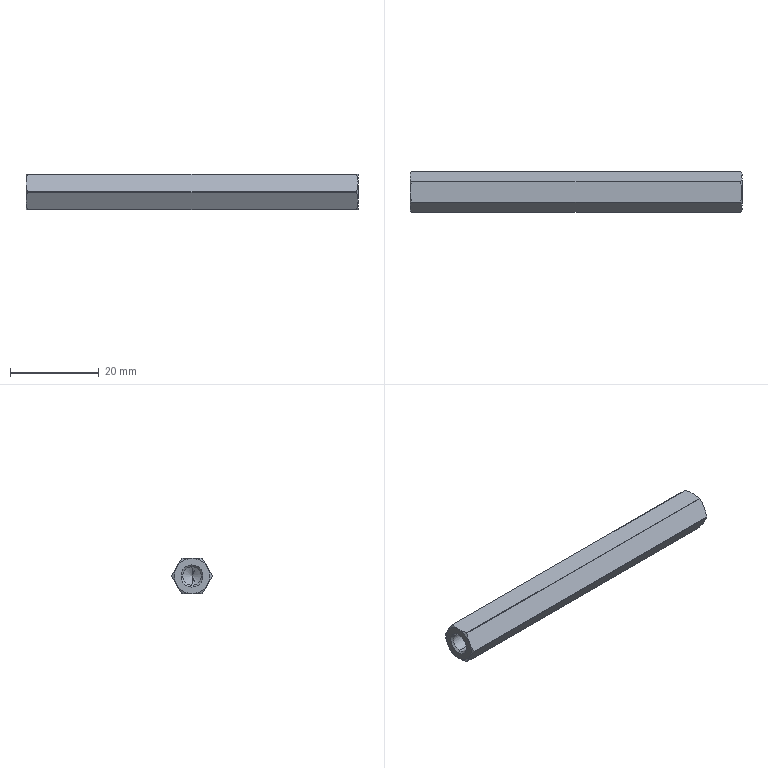Part | STEP file | SceondLSFB8-75 | 1 solid | 38 faces | box 75 x 9.2 x 8 mm | volume 3839 mm3 | cone 20 | cylinder 10 | plane 8 | commonest cylinder face diameters 9.2 x6 4.134 x4
STEP:
#1=CARTESIAN_POINT('',(74.567,0.,2.067));
#2=VERTEX_POINT('',#1);
#3=CARTESIAN_POINT('',(74.567,0.,-2.067));
#4=VERTEX_POINT('',#3);
#5=CARTESIAN_POINT('',(74.567,0.,0.));
#6=DIRECTION('',(1.,0.,0.));
#7=DIRECTION('',(0.,1.,0.));
#8=AXIS2_PLACEMENT_3D('',#5,#6,#7);
#9=CIRCLE('',#8,2.067);
#10=EDGE_CURVE('',#2,#4,#9,.T.);
#11=ORIENTED_EDGE('',*,*,#10,.F.);
#12=CARTESIAN_POINT('',(75.,0.,2.5));
#13=VERTEX_POINT('',#12);
#14=CARTESIAN_POINT('',(75.,0.,2.5));
#15=DIRECTION('',(0.7071,0.,0.7071));
#16=VECTOR('',#15,1000.);
#17=LINE('',#14,#16);
#18=EDGE_CURVE('',#2,#13,#17,.T.);
#19=ORIENTED_EDGE('',*,*,#18,.T.);
#20=CARTESIAN_POINT('',(75.,0.,-2.5));
#21=VERTEX_POINT('',#20);
#22=CARTESIAN_POINT('',(75.,0.,0.));
#23=DIRECTION('',(-1.,0.,0.));
#24=DIRECTION('',(0.,0.,-1.));
#25=AXIS2_PLACEMENT_3D('',#22,#23,#24);
#26=CIRCLE('',#25,2.5);
#27=EDGE_CURVE('',#21,#13,#26,.T.);
#28=ORIENTED_EDGE('',*,*,#27,.F.);
#29=CARTESIAN_POINT('',(75.,0.,-2.5));
#30=DIRECTION('',(0.7071,0.,-0.7071));
#31=VECTOR('',#30,1000.);
#32=LINE('',#29,#31);
#33=EDGE_CURVE('',#4,#21,#32,.T.);
#34=ORIENTED_EDGE('',*,*,#33,.F.);
#35=EDGE_LOOP('',(#11,#19,#28,#34));
#36=FACE_OUTER_BOUND('',#35,.T.);
#37=CARTESIAN_POINT('',(75.,0.,0.));
#38=DIRECTION('',(1.,0.,0.));
#39=DIRECTION('',(0.,0.,-1.));
#40=AXIS2_PLACEMENT_3D('',#37,#38,#39);
#41=CONICAL_SURFACE('',#40,2.5,0.7854);
#42=ADVANCED_FACE('',(#36),#41,.F.);
#43=CARTESIAN_POINT('',(0.433,0.,-2.067));
#44=VERTEX_POINT('',#43);
#45=CARTESIAN_POINT('',(0.433,0.,2.067));
#46=VERTEX_POINT('',#45);
#47=CARTESIAN_POINT('',(0.433,0.,0.));
#48=DIRECTION('',(-1.,0.,0.));
#49=DIRECTION('',(0.,1.,0.));
#50=AXIS2_PLACEMENT_3D('',#47,#48,#49);
#51=CIRCLE('',#50,2.067);
#52=EDGE_CURVE('',#44,#46,#51,.T.);
#53=ORIENTED_EDGE('',*,*,#52,.F.);
#54=CARTESIAN_POINT('',(0.,0.,-2.5));
#55=VERTEX_POINT('',#54);
#56=CARTESIAN_POINT('',(0.,0.,-2.5));
#57=DIRECTION('',(-0.7071,0.,-0.7071));
#58=VECTOR('',#57,1000.);
#59=LINE('',#56,#58);
#60=EDGE_CURVE('',#44,#55,#59,.T.);
#61=ORIENTED_EDGE('',*,*,#60,.T.);
#62=CARTESIAN_POINT('',(0.,0.,2.5));
#63=VERTEX_POINT('',#62);
#64=CARTESIAN_POINT('',(0.,0.,0.));
#65=DIRECTION('',(1.,0.,0.));
#66=DIRECTION('',(0.,0.,1.));
#67=AXIS2_PLACEMENT_3D('',#64,#65,#66);
#68=CIRCLE('',#67,2.5);
#69=EDGE_CURVE('',#63,#55,#68,.T.);
#70=ORIENTED_EDGE('',*,*,#69,.F.);
#71=CARTESIAN_POINT('',(0.,0.,2.5));
#72=DIRECTION('',(-0.7071,0.,0.7071));
#73=VECTOR('',#72,1000.);
#74=LINE('',#71,#73);
#75=EDGE_CURVE('',#46,#63,#74,.T.);
#76=ORIENTED_EDGE('',*,*,#75,.F.);
#77=EDGE_LOOP('',(#53,#61,#70,#76));
#78=FACE_OUTER_BOUND('',#77,.T.);
#79=CARTESIAN_POINT('',(0.,0.,0.));
#80=DIRECTION('',(-1.,0.,0.));
#81=DIRECTION('',(0.,0.,1.));
#82=AXIS2_PLACEMENT_3D('',#79,#80,#81);
#83=CONICAL_SURFACE('',#82,2.5,0.7854);
#84=ADVANCED_FACE('',(#78),#83,.F.);
#85=CARTESIAN_POINT('',(63.693,0.,2.067));
#86=VERTEX_POINT('',#85);
#87=CARTESIAN_POINT('',(63.693,0.,-2.067));
#88=VERTEX_POINT('',#87);
#89=CARTESIAN_POINT('',(63.693,0.,0.));
#90=DIRECTION('',(1.,0.,0.));
#91=DIRECTION('',(0.,0.,-1.));
#92=AXIS2_PLACEMENT_3D('',#89,#90,#91);
#93=CIRCLE('',#92,2.067);
#94=EDGE_CURVE('',#86,#88,#93,.T.);
#95=ORIENTED_EDGE('',*,*,#94,.F.);
#96=CARTESIAN_POINT('',(69.13,0.,2.067));
#97=DIRECTION('',(1.,0.,0.));
#98=VECTOR('',#97,1000.);
#99=LINE('',#96,#98);
#100=EDGE_CURVE('',#86,#2,#99,.T.);
#101=ORIENTED_EDGE('',*,*,#100,.T.);
#102=ORIENTED_EDGE('',*,*,#10,.T.);
#103=CARTESIAN_POINT('',(69.13,0.,-2.067));
#104=DIRECTION('',(1.,0.,0.));
#105=VECTOR('',#104,1000.);
#106=LINE('',#103,#105);
#107=EDGE_CURVE('',#88,#4,#106,.T.);
#108=ORIENTED_EDGE('',*,*,#107,.F.);
#109=EDGE_LOOP('',(#95,#101,#102,#108));
#110=FACE_OUTER_BOUND('',#109,.T.);
#111=CARTESIAN_POINT('',(69.13,0.,0.));
#112=DIRECTION('',(1.,0.,0.));
#113=DIRECTION('',(0.,0.,-1.));
#114=AXIS2_PLACEMENT_3D('',#111,#112,#113);
#115=CYLINDRICAL_SURFACE('',#114,2.067);
#116=ADVANCED_FACE('',(#110),#115,.F.);
#117=ORIENTED_EDGE('',*,*,#52,.T.);
#118=CARTESIAN_POINT('',(11.307,0.,2.067));
#119=VERTEX_POINT('',#118);
#120=CARTESIAN_POINT('',(5.87,0.,2.067));
#121=DIRECTION('',(1.,0.,0.));
#122=VECTOR('',#121,1000.);
#123=LINE('',#120,#122);
#124=EDGE_CURVE('',#46,#119,#123,.T.);
#125=ORIENTED_EDGE('',*,*,#124,.T.);
#126=CARTESIAN_POINT('',(11.307,0.,-2.067));
#127=VERTEX_POINT('',#126);
#128=CARTESIAN_POINT('',(11.307,0.,0.));
#129=DIRECTION('',(-1.,0.,0.));
#130=DIRECTION('',(0.,0.,-1.));
#131=AXIS2_PLACEMENT_3D('',#128,#129,#130);
#132=CIRCLE('',#131,2.067);
#133=EDGE_CURVE('',#127,#119,#132,.T.);
#134=ORIENTED_EDGE('',*,*,#133,.F.);
#135=CARTESIAN_POINT('',(5.87,0.,-2.067));
#136=DIRECTION('',(1.,0.,0.));
#137=VECTOR('',#136,1000.);
#138=LINE('',#135,#137);
#139=EDGE_CURVE('',#44,#127,#138,.T.);
#140=ORIENTED_EDGE('',*,*,#139,.F.);
#141=EDGE_LOOP('',(#117,#125,#134,#140));
#142=FACE_OUTER_BOUND('',#141,.T.);
#143=CARTESIAN_POINT('',(5.87,0.,0.));
#144=DIRECTION('',(1.,0.,0.));
#145=DIRECTION('',(0.,0.,-1.));
#146=AXIS2_PLACEMENT_3D('',#143,#144,#145);
#147=CYLINDRICAL_SURFACE('',#146,2.067);
#148=ADVANCED_FACE('',(#142),#147,.F.);
#149=CARTESIAN_POINT('',(62.5,0.,0.));
#150=VERTEX_POINT('',#149);
#151=CARTESIAN_POINT('',(63.693,0.,-2.067));
#152=DIRECTION('',(0.5,0.,-0.866));
#153=VECTOR('',#152,1000.);
#154=LINE('',#151,#153);
#155=EDGE_CURVE('',#150,#88,#154,.T.);
#156=ORIENTED_EDGE('',*,*,#155,.F.);
#157=CARTESIAN_POINT('',(63.693,0.,2.067));
#158=DIRECTION('',(0.5,0.,0.866));
#159=VECTOR('',#158,1000.);
#160=LINE('',#157,#159);
#161=EDGE_CURVE('',#150,#86,#160,.T.);
#162=ORIENTED_EDGE('',*,*,#161,.T.);
#163=ORIENTED_EDGE('',*,*,#94,.T.);
#164=EDGE_LOOP('',(#156,#162,#163));
#165=FACE_OUTER_BOUND('',#164,.T.);
#166=CARTESIAN_POINT('',(63.693,0.,0.));
#167=DIRECTION('',(1.,0.,0.));
#168=DIRECTION('',(0.,0.,-1.));
#169=AXIS2_PLACEMENT_3D('',#166,#167,#168);
#170=CONICAL_SURFACE('',#169,2.067,1.047);
#171=ADVANCED_FACE('',(#165),#170,.F.);
#172=CARTESIAN_POINT('',(12.5,0.,0.));
#173=VERTEX_POINT('',#172);
#174=CARTESIAN_POINT('',(11.307,0.,2.067));
#175=DIRECTION('',(-0.5,0.,0.866));
#176=VECTOR('',#175,1000.);
#177=LINE('',#174,#176);
#178=EDGE_CURVE('',#173,#119,#177,.T.);
#179=ORIENTED_EDGE('',*,*,#178,.F.);
#180=CARTESIAN_POINT('',(11.307,0.,-2.067));
#181=DIRECTION('',(-0.5,0.,-0.866));
#182=VECTOR('',#181,1000.);
#183=LINE('',#180,#182);
#184=EDGE_CURVE('',#173,#127,#183,.T.);
#185=ORIENTED_EDGE('',*,*,#184,.T.);
#186=ORIENTED_EDGE('',*,*,#133,.T.);
#187=EDGE_LOOP('',(#179,#185,#186));
#188=FACE_OUTER_BOUND('',#187,.T.);
#189=CARTESIAN_POINT('',(11.307,0.,0.));
#190=DIRECTION('',(-1.,0.,0.));
#191=DIRECTION('',(0.,0.,1.));
#192=AXIS2_PLACEMENT_3D('',#189,#190,#191);
#193=CONICAL_SURFACE('',#192,2.067,1.047);
#194=ADVANCED_FACE('',(#188),#193,.F.);
#195=CARTESIAN_POINT('',(74.654,2.328,-3.967));
#196=VERTEX_POINT('',#195);
#197=CARTESIAN_POINT('',(75.,3.464,-2.));
#198=VERTEX_POINT('',#197);
#199=CARTESIAN_POINT('',(74.654,2.328,-3.967));
#200=CARTESIAN_POINT('',(74.865,2.7,-3.324));
#201=CARTESIAN_POINT('',(75.,3.077,-2.671));
#202=CARTESIAN_POINT('',(75.,3.464,-2.));
#203=B_SPLINE_CURVE_WITH_KNOTS('',3,(#199,#200,#201,#202),.UNSPECIFIED.,.F.,.F.,(4,4),(0.,0.002298),.UNSPECIFIED.);
#204=EDGE_CURVE('',#196,#198,#203,.T.);
#205=ORIENTED_EDGE('',*,*,#204,.F.);
#206=CARTESIAN_POINT('',(0.3464,2.328,-3.967));
#207=VERTEX_POINT('',#206);
#208=CARTESIAN_POINT('',(0.,2.328,-3.967));
#209=DIRECTION('',(1.,0.,0.));
#210=VECTOR('',#209,1000.);
#211=LINE('',#208,#210);
#212=EDGE_CURVE('',#207,#196,#211,.T.);
#213=ORIENTED_EDGE('',*,*,#212,.F.);
#214=CARTESIAN_POINT('',(0.,3.464,-2.));
#215=VERTEX_POINT('',#214);
#216=CARTESIAN_POINT('',(0.,3.464,-2.));
#217=CARTESIAN_POINT('',(0.,3.077,-2.671));
#218=CARTESIAN_POINT('',(0.1347,2.7,-3.324));
#219=CARTESIAN_POINT('',(0.3464,2.328,-3.967));
#220=B_SPLINE_CURVE_WITH_KNOTS('',3,(#216,#217,#218,#219),.UNSPECIFIED.,.F.,.F.,(4,4),(0.,0.002298),.UNSPECIFIED.);
#221=EDGE_CURVE('',#215,#207,#220,.T.);
#222=ORIENTED_EDGE('',*,*,#221,.F.);
#223=CARTESIAN_POINT('',(0.3464,4.6,-0.03277));
#224=VERTEX_POINT('',#223);
#225=CARTESIAN_POINT('',(0.3464,4.6,-0.03277));
#226=CARTESIAN_POINT('',(0.1347,4.229,-0.6758));
#227=CARTESIAN_POINT('',(0.,3.852,-1.329));
#228=CARTESIAN_POINT('',(0.,3.464,-2.));
#229=B_SPLINE_CURVE_WITH_KNOTS('',3,(#225,#226,#227,#228),.UNSPECIFIED.,.F.,.F.,(4,4),(0.,0.002298),.UNSPECIFIED.);
#230=EDGE_CURVE('',#224,#215,#229,.T.);
#231=ORIENTED_EDGE('',*,*,#230,.F.);
#232=CARTESIAN_POINT('',(74.654,4.6,-0.03277));
#233=VERTEX_POINT('',#232);
#234=CARTESIAN_POINT('',(0.,4.6,-0.03277));
#235=DIRECTION('',(-1.,0.,0.));
#236=VECTOR('',#235,1000.);
#237=LINE('',#234,#236);
#238=EDGE_CURVE('',#233,#224,#237,.T.);
#239=ORIENTED_EDGE('',*,*,#238,.F.);
#240=CARTESIAN_POINT('',(75.,3.464,-2.));
#241=CARTESIAN_POINT('',(75.,3.852,-1.329));
#242=CARTESIAN_POINT('',(74.865,4.229,-0.6758));
#243=CARTESIAN_POINT('',(74.654,4.6,-0.03277));
#244=B_SPLINE_CURVE_WITH_KNOTS('',3,(#240,#241,#242,#243),.UNSPECIFIED.,.F.,.F.,(4,4),(0.,0.002298),.UNSPECIFIED.);
#245=EDGE_CURVE('',#198,#233,#244,.T.);
#246=ORIENTED_EDGE('',*,*,#245,.F.);
#247=EDGE_LOOP('',(#205,#213,#222,#231,#239,#246));
#248=FACE_OUTER_BOUND('',#247,.T.);
#249=CARTESIAN_POINT('',(0.,2.309,-4.));
#250=DIRECTION('',(0.,-0.866,0.5));
#251=DIRECTION('',(0.,-0.5,-0.866));
#252=AXIS2_PLACEMENT_3D('',#249,#250,#251);
#253=PLANE('',#252);
#254=ADVANCED_FACE('',(#248),#253,.F.);
#255=ORIENTED_EDGE('',*,*,#245,.T.);
#256=CARTESIAN_POINT('',(74.654,4.6,0.03277));
#257=VERTEX_POINT('',#256);
#258=CARTESIAN_POINT('',(74.654,0.,0.));
#259=DIRECTION('',(1.,0.,0.));
#260=DIRECTION('',(0.,1.,0.));
#261=AXIS2_PLACEMENT_3D('',#258,#259,#260);
#262=CIRCLE('',#261,4.6);
#263=EDGE_CURVE('',#233,#257,#262,.T.);
#264=ORIENTED_EDGE('',*,*,#263,.T.);
#265=CARTESIAN_POINT('',(75.,3.464,2.));
#266=VERTEX_POINT('',#265);
#267=CARTESIAN_POINT('',(74.654,4.6,0.03277));
#268=CARTESIAN_POINT('',(74.865,4.229,0.6758));
#269=CARTESIAN_POINT('',(75.,3.852,1.329));
#270=CARTESIAN_POINT('',(75.,3.464,2.));
#271=B_SPLINE_CURVE_WITH_KNOTS('',3,(#267,#268,#269,#270),.UNSPECIFIED.,.F.,.F.,(4,4),(0.,0.002298),.UNSPECIFIED.);
#272=EDGE_CURVE('',#257,#266,#271,.T.);
#273=ORIENTED_EDGE('',*,*,#272,.T.);
#274=CARTESIAN_POINT('',(75.,0.,0.));
#275=DIRECTION('',(-1.,0.,0.));
#276=DIRECTION('',(0.,0.,1.));
#277=AXIS2_PLACEMENT_3D('',#274,#275,#276);
#278=CIRCLE('',#277,4.);
#279=EDGE_CURVE('',#266,#198,#278,.T.);
#280=ORIENTED_EDGE('',*,*,#279,.T.);
#281=EDGE_LOOP('',(#255,#264,#273,#280));
#282=FACE_OUTER_BOUND('',#281,.T.);
#283=CARTESIAN_POINT('',(74.654,0.,0.));
#284=DIRECTION('',(-1.,0.,0.));
#285=DIRECTION('',(0.,0.,1.));
#286=AXIS2_PLACEMENT_3D('',#283,#284,#285);
#287=CONICAL_SURFACE('',#286,4.6,1.047);
#288=ADVANCED_FACE('',(#282),#287,.T.);
#289=ORIENTED_EDGE('',*,*,#204,.T.);
#290=CARTESIAN_POINT('',(75.,0.,-4.));
#291=VERTEX_POINT('',#290);
#292=CARTESIAN_POINT('',(75.,0.,0.));
#293=DIRECTION('',(-1.,0.,0.));
#294=DIRECTION('',(0.,0.,1.));
#295=AXIS2_PLACEMENT_3D('',#292,#293,#294);
#296=CIRCLE('',#295,4.);
#297=EDGE_CURVE('',#198,#291,#296,.T.);
#298=ORIENTED_EDGE('',*,*,#297,.T.);
#299=CARTESIAN_POINT('',(74.654,2.272,-4.));
#300=VERTEX_POINT('',#299);
#301=CARTESIAN_POINT('',(75.,0.,-4.));
#302=CARTESIAN_POINT('',(75.,0.7748,-4.));
#303=CARTESIAN_POINT('',(74.865,1.529,-4.));
#304=CARTESIAN_POINT('',(74.654,2.272,-4.));
#305=B_SPLINE_CURVE_WITH_KNOTS('',3,(#301,#302,#303,#304),.UNSPECIFIED.,.F.,.F.,(4,4),(0.,0.002298),.UNSPECIFIED.);
#306=EDGE_CURVE('',#291,#300,#305,.T.);
#307=ORIENTED_EDGE('',*,*,#306,.T.);
#308=CARTESIAN_POINT('',(74.654,0.,0.));
#309=DIRECTION('',(1.,0.,0.));
#310=DIRECTION('',(0.,1.,0.));
#311=AXIS2_PLACEMENT_3D('',#308,#309,#310);
#312=CIRCLE('',#311,4.6);
#313=EDGE_CURVE('',#300,#196,#312,.T.);
#314=ORIENTED_EDGE('',*,*,#313,.T.);
#315=EDGE_LOOP('',(#289,#298,#307,#314));
#316=FACE_OUTER_BOUND('',#315,.T.);
#317=CARTESIAN_POINT('',(74.654,0.,0.));
#318=DIRECTION('',(-1.,0.,0.));
#319=DIRECTION('',(0.,0.,1.));
#320=AXIS2_PLACEMENT_3D('',#317,#318,#319);
#321=CONICAL_SURFACE('',#320,4.6,1.047);
#322=ADVANCED_FACE('',(#316),#321,.T.);
#323=ORIENTED_EDGE('',*,*,#212,.T.);
#324=ORIENTED_EDGE('',*,*,#313,.F.);
#325=CARTESIAN_POINT('',(0.3464,2.272,-4.));
#326=VERTEX_POINT('',#325);
#327=CARTESIAN_POINT('',(37.5,2.272,-4.));
#328=DIRECTION('',(-1.,0.,0.));
#329=VECTOR('',#328,1000.);
#330=LINE('',#327,#329);
#331=EDGE_CURVE('',#300,#326,#330,.T.);
#332=ORIENTED_EDGE('',*,*,#331,.T.);
#333=CARTESIAN_POINT('',(0.3464,0.,0.));
#334=DIRECTION('',(1.,0.,0.));
#335=DIRECTION('',(0.,0.,-1.));
#336=AXIS2_PLACEMENT_3D('',#333,#334,#335);
#337=CIRCLE('',#336,4.6);
#338=EDGE_CURVE('',#326,#207,#337,.T.);
#339=ORIENTED_EDGE('',*,*,#338,.T.);
#340=EDGE_LOOP('',(#323,#324,#332,#339));
#341=FACE_OUTER_BOUND('',#340,.T.);
#342=CARTESIAN_POINT('',(37.5,0.,0.));
#343=DIRECTION('',(1.,0.,0.));
#344=DIRECTION('',(0.,0.,-1.));
#345=AXIS2_PLACEMENT_3D('',#342,#343,#344);
#346=CYLINDRICAL_SURFACE('',#345,4.6);
#347=ADVANCED_FACE('',(#341),#346,.T.);
#348=ORIENTED_EDGE('',*,*,#221,.T.);
#349=ORIENTED_EDGE('',*,*,#338,.F.);
#350=CARTESIAN_POINT('',(0.,0.,-4.));
#351=VERTEX_POINT('',#350);
#352=CARTESIAN_POINT('',(0.3464,2.272,-4.));
#353=CARTESIAN_POINT('',(0.1347,1.529,-4.));
#354=CARTESIAN_POINT('',(0.,0.7748,-4.));
#355=CARTESIAN_POINT('',(0.,0.,-4.));
#356=B_SPLINE_CURVE_WITH_KNOTS('',3,(#352,#353,#354,#355),.UNSPECIFIED.,.F.,.F.,(4,4),(0.,0.002298),.UNSPECIFIED.);
#357=EDGE_CURVE('',#326,#351,#356,.T.);
#358=ORIENTED_EDGE('',*,*,#357,.T.);
#359=CARTESIAN_POINT('',(0.,0.,0.));
#360=DIRECTION('',(1.,0.,0.));
#361=DIRECTION('',(0.,0.,-1.));
#362=AXIS2_PLACEMENT_3D('',#359,#360,#361);
#363=CIRCLE('',#362,4.);
#364=EDGE_CURVE('',#351,#215,#363,.T.);
#365=ORIENTED_EDGE('',*,*,#364,.T.);
#366=EDGE_LOOP('',(#348,#349,#358,#365));
#367=FACE_OUTER_BOUND('',#366,.T.);
#368=CARTESIAN_POINT('',(0.3464,0.,0.));
#369=DIRECTION('',(1.,0.,0.));
#370=DIRECTION('',(0.,0.,-1.));
#371=AXIS2_PLACEMENT_3D('',#368,#369,#370);
#372=CONICAL_SURFACE('',#371,4.6,1.047);
#373=ADVANCED_FACE('',(#367),#372,.T.);
#374=ORIENTED_EDGE('',*,*,#230,.T.);
#375=CARTESIAN_POINT('',(0.,3.464,2.));
#376=VERTEX_POINT('',#375);
#377=CARTESIAN_POINT('',(0.,0.,0.));
#378=DIRECTION('',(1.,0.,0.));
#379=DIRECTION('',(0.,0.,-1.));
#380=AXIS2_PLACEMENT_3D('',#377,#378,#379);
#381=CIRCLE('',#380,4.);
#382=EDGE_CURVE('',#215,#376,#381,.T.);
#383=ORIENTED_EDGE('',*,*,#382,.T.);
#384=CARTESIAN_POINT('',(0.3464,4.6,0.03277));
#385=VERTEX_POINT('',#384);
#386=CARTESIAN_POINT('',(0.,3.464,2.));
#387=CARTESIAN_POINT('',(0.,3.852,1.329));
#388=CARTESIAN_POINT('',(0.1347,4.229,0.6758));
#389=CARTESIAN_POINT('',(0.3464,4.6,0.03277));
#390=B_SPLINE_CURVE_WITH_KNOTS('',3,(#386,#387,#388,#389),.UNSPECIFIED.,.F.,.F.,(4,4),(0.,0.002298),.UNSPECIFIED.);
#391=EDGE_CURVE('',#376,#385,#390,.T.);
#392=ORIENTED_EDGE('',*,*,#391,.T.);
#393=CARTESIAN_POINT('',(0.3464,0.,0.));
#394=DIRECTION('',(-1.,0.,0.));
#395=DIRECTION('',(0.,1.,0.));
#396=AXIS2_PLACEMENT_3D('',#393,#394,#395);
#397=CIRCLE('',#396,4.6);
#398=EDGE_CURVE('',#385,#224,#397,.T.);
#399=ORIENTED_EDGE('',*,*,#398,.T.);
#400=EDGE_LOOP('',(#374,#383,#392,#399));
#401=FACE_OUTER_BOUND('',#400,.T.);
#402=CARTESIAN_POINT('',(0.3464,0.,0.));
#403=DIRECTION('',(1.,0.,0.));
#404=DIRECTION('',(0.,0.,-1.));
#405=AXIS2_PLACEMENT_3D('',#402,#403,#404);
#406=CONICAL_SURFACE('',#405,4.6,1.047);
#407=ADVANCED_FACE('',(#401),#406,.T.);
#408=ORIENTED_EDGE('',*,*,#238,.T.);
#409=ORIENTED_EDGE('',*,*,#398,.F.);
#410=CARTESIAN_POINT('',(37.5,4.6,0.03277));
#411=DIRECTION('',(1.,0.,0.));
#412=VECTOR('',#411,1000.);
#413=LINE('',#410,#412);
#414=EDGE_CURVE('',#385,#257,#413,.T.);
#415=ORIENTED_EDGE('',*,*,#414,.T.);
#416=ORIENTED_EDGE('',*,*,#263,.F.);
#417=EDGE_LOOP('',(#408,#409,#415,#416));
#418=FACE_OUTER_BOUND('',#417,.T.);
#419=CARTESIAN_POINT('',(37.5,0.,0.));
#420=DIRECTION('',(1.,0.,0.));
#421=DIRECTION('',(0.,0.,-1.));
#422=AXIS2_PLACEMENT_3D('',#419,#420,#421);
#423=CYLINDRICAL_SURFACE('',#422,4.6);
#424=ADVANCED_FACE('',(#418),#423,.T.);
#425=ORIENTED_EDGE('',*,*,#297,.F.);
#426=ORIENTED_EDGE('',*,*,#279,.F.);
#427=CARTESIAN_POINT('',(75.,0.,4.));
#428=VERTEX_POINT('',#427);
#429=CARTESIAN_POINT('',(75.,0.,0.));
#430=DIRECTION('',(1.,0.,0.));
#431=DIRECTION('',(0.,0.,1.));
#432=AXIS2_PLACEMENT_3D('',#429,#430,#431);
#433=CIRCLE('',#432,4.);
#434=EDGE_CURVE('',#266,#428,#433,.T.);
#435=ORIENTED_EDGE('',*,*,#434,.T.);
#436=CARTESIAN_POINT('',(75.,-3.464,2.));
#437=VERTEX_POINT('',#436);
#438=CARTESIAN_POINT('',(75.,0.,0.));
#439=DIRECTION('',(1.,0.,0.));
#440=DIRECTION('',(0.,0.,1.));
#441=AXIS2_PLACEMENT_3D('',#438,#439,#440);
#442=CIRCLE('',#441,4.);
#443=EDGE_CURVE('',#428,#437,#442,.T.);
#444=ORIENTED_EDGE('',*,*,#443,.T.);
#445=CARTESIAN_POINT('',(75.,-3.464,-2.));
#446=VERTEX_POINT('',#445);
#447=CARTESIAN_POINT('',(75.,0.,0.));
#448=DIRECTION('',(1.,0.,0.));
#449=DIRECTION('',(0.,0.,1.));
#450=AXIS2_PLACEMENT_3D('',#447,#448,#449);
#451=CIRCLE('',#450,4.);
#452=EDGE_CURVE('',#437,#446,#451,.T.);
#453=ORIENTED_EDGE('',*,*,#452,.T.);
#454=CARTESIAN_POINT('',(75.,0.,0.));
#455=DIRECTION('',(1.,0.,0.));
#456=DIRECTION('',(0.,0.,1.));
#457=AXIS2_PLACEMENT_3D('',#454,#455,#456);
#458=CIRCLE('',#457,4.);
#459=EDGE_CURVE('',#446,#291,#458,.T.);
#460=ORIENTED_EDGE('',*,*,#459,.T.);
#461=EDGE_LOOP('',(#425,#426,#435,#444,#453,#460));
#462=FACE_OUTER_BOUND('',#461,.T.);
#463=ORIENTED_EDGE('',*,*,#27,.T.);
#464=CARTESIAN_POINT('',(75.,0.,0.));
#465=DIRECTION('',(-1.,0.,0.));
#466=DIRECTION('',(0.,0.,-1.));
#467=AXIS2_PLACEMENT_3D('',#464,#465,#466);
#468=CIRCLE('',#467,2.5);
#469=EDGE_CURVE('',#13,#21,#468,.T.);
#470=ORIENTED_EDGE('',*,*,#469,.T.);
#471=EDGE_LOOP('',(#463,#470));
#472=FACE_BOUND('',#471,.T.);
#473=CARTESIAN_POINT('',(75.,2.,0.));
#474=DIRECTION('',(1.,0.,0.));
#475=DIRECTION('',(0.,0.,-1.));
#476=AXIS2_PLACEMENT_3D('',#473,#474,#475);
#477=PLANE('',#476);
#478=ADVANCED_FACE('',(#462,#472),#477,.T.);
#479=CARTESIAN_POINT('',(74.654,-2.272,-4.));
#480=VERTEX_POINT('',#479);
#481=CARTESIAN_POINT('',(74.654,-2.272,-4.));
#482=CARTESIAN_POINT('',(74.865,-1.529,-4.));
#483=CARTESIAN_POINT('',(75.,-0.7748,-4.));
#484=CARTESIAN_POINT('',(75.,0.,-4.));
#485=B_SPLINE_CURVE_WITH_KNOTS('',3,(#481,#482,#483,#484),.UNSPECIFIED.,.F.,.F.,(4,4),(0.,0.002298),.UNSPECIFIED.);
#486=EDGE_CURVE('',#480,#291,#485,.T.);
#487=ORIENTED_EDGE('',*,*,#486,.F.);
#488=CARTESIAN_POINT('',(0.3464,-2.272,-4.));
#489=VERTEX_POINT('',#488);
#490=CARTESIAN_POINT('',(0.,-2.272,-4.));
#491=DIRECTION('',(1.,0.,0.));
#492=VECTOR('',#491,1000.);
#493=LINE('',#490,#492);
#494=EDGE_CURVE('',#489,#480,#493,.T.);
#495=ORIENTED_EDGE('',*,*,#494,.F.);
#496=CARTESIAN_POINT('',(0.,0.,-4.));
#497=CARTESIAN_POINT('',(0.,-0.7748,-4.));
#498=CARTESIAN_POINT('',(0.1347,-1.529,-4.));
#499=CARTESIAN_POINT('',(0.3464,-2.272,-4.));
#500=B_SPLINE_CURVE_WITH_KNOTS('',3,(#496,#497,#498,#499),.UNSPECIFIED.,.F.,.F.,(4,4),(0.,0.002298),.UNSPECIFIED.);
#501=EDGE_CURVE('',#351,#489,#500,.T.);
#502=ORIENTED_EDGE('',*,*,#501,.F.);
#503=ORIENTED_EDGE('',*,*,#357,.F.);
#504=ORIENTED_EDGE('',*,*,#331,.F.);
#505=ORIENTED_EDGE('',*,*,#306,.F.);
#506=EDGE_LOOP('',(#487,#495,#502,#503,#504,#505));
#507=FACE_OUTER_BOUND('',#506,.T.);
#508=CARTESIAN_POINT('',(0.,-2.309,-4.));
#509=DIRECTION('',(0.,0.,1.));
#510=DIRECTION('',(1.,0.,0.));
#511=AXIS2_PLACEMENT_3D('',#508,#509,#510);
#512=PLANE('',#511);
#513=ADVANCED_FACE('',(#507),#512,.F.);
#514=CARTESIAN_POINT('',(0.,-3.464,2.));
#515=VERTEX_POINT('',#514);
#516=CARTESIAN_POINT('',(0.,0.,4.));
#517=VERTEX_POINT('',#516);
#518=CARTESIAN_POINT('',(0.,0.,0.));
#519=DIRECTION('',(-1.,0.,0.));
#520=DIRECTION('',(0.,0.,-1.));
#521=AXIS2_PLACEMENT_3D('',#518,#519,#520);
#522=CIRCLE('',#521,4.);
#523=EDGE_CURVE('',#515,#517,#522,.T.);
#524=ORIENTED_EDGE('',*,*,#523,.T.);
#525=CARTESIAN_POINT('',(0.,0.,0.));
#526=DIRECTION('',(-1.,0.,0.));
#527=DIRECTION('',(0.,0.,-1.));
#528=AXIS2_PLACEMENT_3D('',#525,#526,#527);
#529=CIRCLE('',#528,4.);
#530=EDGE_CURVE('',#517,#376,#529,.T.);
#531=ORIENTED_EDGE('',*,*,#530,.T.);
#532=ORIENTED_EDGE('',*,*,#382,.F.);
#533=ORIENTED_EDGE('',*,*,#364,.F.);
#534=CARTESIAN_POINT('',(0.,-3.464,-2.));
#535=VERTEX_POINT('',#534);
#536=CARTESIAN_POINT('',(0.,0.,0.));
#537=DIRECTION('',(-1.,0.,0.));
#538=DIRECTION('',(0.,0.,-1.));
#539=AXIS2_PLACEMENT_3D('',#536,#537,#538);
#540=CIRCLE('',#539,4.);
#541=EDGE_CURVE('',#351,#535,#540,.T.);
#542=ORIENTED_EDGE('',*,*,#541,.T.);
#543=CARTESIAN_POINT('',(0.,0.,0.));
#544=DIRECTION('',(-1.,0.,0.));
#545=DIRECTION('',(0.,0.,-1.));
#546=AXIS2_PLACEMENT_3D('',#543,#544,#545);
#547=CIRCLE('',#546,4.);
#548=EDGE_CURVE('',#535,#515,#547,.T.);
#549=ORIENTED_EDGE('',*,*,#548,.T.);
#550=EDGE_LOOP('',(#524,#531,#532,#533,#542,#549));
#551=FACE_OUTER_BOUND('',#550,.T.);
#552=ORIENTED_EDGE('',*,*,#69,.T.);
#553=CARTESIAN_POINT('',(0.,0.,0.));
#554=DIRECTION('',(1.,0.,0.));
#555=DIRECTION('',(0.,0.,1.));
#556=AXIS2_PLACEMENT_3D('',#553,#554,#555);
#557=CIRCLE('',#556,2.5);
#558=EDGE_CURVE('',#55,#63,#557,.T.);
#559=ORIENTED_EDGE('',*,*,#558,.T.);
#560=EDGE_LOOP('',(#552,#559));
#561=FACE_BOUND('',#560,.T.);
#562=CARTESIAN_POINT('',(0.,2.,0.));
#563=DIRECTION('',(-1.,0.,0.));
#564=DIRECTION('',(0.,0.,1.));
#565=AXIS2_PLACEMENT_3D('',#562,#563,#564);
#566=PLANE('',#565);
#567=ADVANCED_FACE('',(#551,#561),#566,.T.);
#568=ORIENTED_EDGE('',*,*,#486,.T.);
#569=ORIENTED_EDGE('',*,*,#459,.F.);
#570=CARTESIAN_POINT('',(74.654,-2.328,-3.967));
#571=VERTEX_POINT('',#570);
#572=CARTESIAN_POINT('',(75.,-3.464,-2.));
#573=CARTESIAN_POINT('',(75.,-3.077,-2.671));
#574=CARTESIAN_POINT('',(74.865,-2.7,-3.324));
#575=CARTESIAN_POINT('',(74.654,-2.328,-3.967));
#576=B_SPLINE_CURVE_WITH_KNOTS('',3,(#572,#573,#574,#575),.UNSPECIFIED.,.F.,.F.,(4,4),(0.,0.002298),.UNSPECIFIED.);
#577=EDGE_CURVE('',#446,#571,#576,.T.);
#578=ORIENTED_EDGE('',*,*,#577,.T.);
#579=CARTESIAN_POINT('',(74.654,0.,0.));
#580=DIRECTION('',(1.,0.,0.));
#581=DIRECTION('',(0.,1.,0.));
#582=AXIS2_PLACEMENT_3D('',#579,#580,#581);
#583=CIRCLE('',#582,4.6);
#584=EDGE_CURVE('',#571,#480,#583,.T.);
#585=ORIENTED_EDGE('',*,*,#584,.T.);
#586=EDGE_LOOP('',(#568,#569,#578,#585));
#587=FACE_OUTER_BOUND('',#586,.T.);
#588=CARTESIAN_POINT('',(74.654,0.,0.));
#589=DIRECTION('',(-1.,0.,0.));
#590=DIRECTION('',(0.,0.,1.));
#591=AXIS2_PLACEMENT_3D('',#588,#589,#590);
#592=CONICAL_SURFACE('',#591,4.6,1.047);
#593=ADVANCED_FACE('',(#587),#592,.T.);
#594=CARTESIAN_POINT('',(74.654,-4.6,-0.03277));
#595=VERTEX_POINT('',#594);
#596=CARTESIAN_POINT('',(74.654,-4.6,-0.03277));
#597=CARTESIAN_POINT('',(74.865,-4.229,-0.6758));
#598=CARTESIAN_POINT('',(75.,-3.852,-1.329));
#599=CARTESIAN_POINT('',(75.,-3.464,-2.));
#600=B_SPLINE_CURVE_WITH_KNOTS('',3,(#596,#597,#598,#599),.UNSPECIFIED.,.F.,.F.,(4,4),(0.,0.002298),.UNSPECIFIED.);
#601=EDGE_CURVE('',#595,#446,#600,.T.);
#602=ORIENTED_EDGE('',*,*,#601,.T.);
#603=ORIENTED_EDGE('',*,*,#452,.F.);
#604=CARTESIAN_POINT('',(74.654,-4.6,0.03277));
#605=VERTEX_POINT('',#604);
#606=CARTESIAN_POINT('',(75.,-3.464,2.));
#607=CARTESIAN_POINT('',(75.,-3.852,1.329));
#608=CARTESIAN_POINT('',(74.865,-4.229,0.6758));
#609=CARTESIAN_POINT('',(74.654,-4.6,0.03277));
#610=B_SPLINE_CURVE_WITH_KNOTS('',3,(#606,#607,#608,#609),.UNSPECIFIED.,.F.,.F.,(4,4),(0.,0.002298),.UNSPECIFIED.);
#611=EDGE_CURVE('',#437,#605,#610,.T.);
#612=ORIENTED_EDGE('',*,*,#611,.T.);
#613=CARTESIAN_POINT('',(74.654,0.,0.));
#614=DIRECTION('',(-1.,0.,0.));
#615=DIRECTION('',(0.,0.,-1.));
#616=AXIS2_PLACEMENT_3D('',#613,#614,#615);
#617=CIRCLE('',#616,4.6);
#618=EDGE_CURVE('',#595,#605,#617,.T.);
#619=ORIENTED_EDGE('',*,*,#618,.F.);
#620=EDGE_LOOP('',(#602,#603,#612,#619));
#621=FACE_OUTER_BOUND('',#620,.T.);
#622=CARTESIAN_POINT('',(74.654,0.,0.));
#623=DIRECTION('',(-1.,0.,0.));
#624=DIRECTION('',(0.,0.,1.));
#625=AXIS2_PLACEMENT_3D('',#622,#623,#624);
#626=CONICAL_SURFACE('',#625,4.6,1.047);
#627=ADVANCED_FACE('',(#621),#626,.T.);
#628=CARTESIAN_POINT('',(74.654,-2.328,3.967));
#629=VERTEX_POINT('',#628);
#630=CARTESIAN_POINT('',(74.654,-2.328,3.967));
#631=CARTESIAN_POINT('',(74.865,-2.7,3.324));
#632=CARTESIAN_POINT('',(75.,-3.077,2.671));
#633=CARTESIAN_POINT('',(75.,-3.464,2.));
#634=B_SPLINE_CURVE_WITH_KNOTS('',3,(#630,#631,#632,#633),.UNSPECIFIED.,.F.,.F.,(4,4),(0.,0.002298),.UNSPECIFIED.);
#635=EDGE_CURVE('',#629,#437,#634,.T.);
#636=ORIENTED_EDGE('',*,*,#635,.T.);
#637=ORIENTED_EDGE('',*,*,#443,.F.);
#638=CARTESIAN_POINT('',(74.654,-2.272,4.));
#639=VERTEX_POINT('',#638);
#640=CARTESIAN_POINT('',(75.,0.,4.));
#641=CARTESIAN_POINT('',(75.,-0.7748,4.));
#642=CARTESIAN_POINT('',(74.865,-1.529,4.));
#643=CARTESIAN_POINT('',(74.654,-2.272,4.));
#644=B_SPLINE_CURVE_WITH_KNOTS('',3,(#640,#641,#642,#643),.UNSPECIFIED.,.F.,.F.,(4,4),(0.,0.002298),.UNSPECIFIED.);
#645=EDGE_CURVE('',#428,#639,#644,.T.);
#646=ORIENTED_EDGE('',*,*,#645,.T.);
#647=CARTESIAN_POINT('',(74.654,0.,0.));
#648=DIRECTION('',(-1.,0.,0.));
#649=DIRECTION('',(0.,0.,-1.));
#650=AXIS2_PLACEMENT_3D('',#647,#648,#649);
#651=CIRCLE('',#650,4.6);
#652=EDGE_CURVE('',#629,#639,#651,.T.);
#653=ORIENTED_EDGE('',*,*,#652,.F.);
#654=EDGE_LOOP('',(#636,#637,#646,#653));
#655=FACE_OUTER_BOUND('',#654,.T.);
#656=CARTESIAN_POINT('',(74.654,0.,0.));
#657=DIRECTION('',(-1.,0.,0.));
#658=DIRECTION('',(0.,0.,1.));
#659=AXIS2_PLACEMENT_3D('',#656,#657,#658);
#660=CONICAL_SURFACE('',#659,4.6,1.047);
#661=ADVANCED_FACE('',(#655),#660,.T.);
#662=CARTESIAN_POINT('',(74.654,2.328,3.967));
#663=VERTEX_POINT('',#662);
#664=CARTESIAN_POINT('',(75.,3.464,2.));
#665=CARTESIAN_POINT('',(75.,3.077,2.671));
#666=CARTESIAN_POINT('',(74.865,2.7,3.324));
#667=CARTESIAN_POINT('',(74.654,2.328,3.967));
#668=B_SPLINE_CURVE_WITH_KNOTS('',3,(#664,#665,#666,#667),.UNSPECIFIED.,.F.,.F.,(4,4),(0.,0.002298),.UNSPECIFIED.);
#669=EDGE_CURVE('',#266,#663,#668,.T.);
#670=ORIENTED_EDGE('',*,*,#669,.T.);
#671=CARTESIAN_POINT('',(74.654,2.272,4.));
#672=VERTEX_POINT('',#671);
#673=CARTESIAN_POINT('',(74.654,0.,0.));
#674=DIRECTION('',(-1.,0.,0.));
#675=DIRECTION('',(0.,0.,-1.));
#676=AXIS2_PLACEMENT_3D('',#673,#674,#675);
#677=CIRCLE('',#676,4.6);
#678=EDGE_CURVE('',#672,#663,#677,.T.);
#679=ORIENTED_EDGE('',*,*,#678,.F.);
#680=CARTESIAN_POINT('',(74.654,2.272,4.));
#681=CARTESIAN_POINT('',(74.865,1.529,4.));
#682=CARTESIAN_POINT('',(75.,0.7748,4.));
#683=CARTESIAN_POINT('',(75.,0.,4.));
#684=B_SPLINE_CURVE_WITH_KNOTS('',3,(#680,#681,#682,#683),.UNSPECIFIED.,.F.,.F.,(4,4),(0.,0.002298),.UNSPECIFIED.);
#685=EDGE_CURVE('',#672,#428,#684,.T.);
#686=ORIENTED_EDGE('',*,*,#685,.T.);
#687=ORIENTED_EDGE('',*,*,#434,.F.);
#688=EDGE_LOOP('',(#670,#679,#686,#687));
#689=FACE_OUTER_BOUND('',#688,.T.);
#690=CARTESIAN_POINT('',(74.654,0.,0.));
#691=DIRECTION('',(-1.,0.,0.));
#692=DIRECTION('',(0.,0.,1.));
#693=AXIS2_PLACEMENT_3D('',#690,#691,#692);
#694=CONICAL_SURFACE('',#693,4.6,1.047);
#695=ADVANCED_FACE('',(#689),#694,.T.);
#696=ORIENTED_EDGE('',*,*,#18,.F.);
#697=CARTESIAN_POINT('',(74.567,0.,0.));
#698=DIRECTION('',(1.,0.,0.));
#699=DIRECTION('',(0.,1.,0.));
#700=AXIS2_PLACEMENT_3D('',#697,#698,#699);
#701=CIRCLE('',#700,2.067);
#702=EDGE_CURVE('',#4,#2,#701,.T.);
#703=ORIENTED_EDGE('',*,*,#702,.F.);
#704=ORIENTED_EDGE('',*,*,#33,.T.);
#705=ORIENTED_EDGE('',*,*,#469,.F.);
#706=EDGE_LOOP('',(#696,#703,#704,#705));
#707=FACE_OUTER_BOUND('',#706,.T.);
#708=CARTESIAN_POINT('',(75.,0.,0.));
#709=DIRECTION('',(1.,0.,0.));
#710=DIRECTION('',(0.,0.,-1.));
#711=AXIS2_PLACEMENT_3D('',#708,#709,#710);
#712=CONICAL_SURFACE('',#711,2.5,0.7854);
#713=ADVANCED_FACE('',(#707),#712,.F.);
#714=ORIENTED_EDGE('',*,*,#494,.T.);
#715=ORIENTED_EDGE('',*,*,#584,.F.);
#716=CARTESIAN_POINT('',(0.3464,-2.328,-3.967));
#717=VERTEX_POINT('',#716);
#718=CARTESIAN_POINT('',(37.5,-2.328,-3.967));
#719=DIRECTION('',(-1.,0.,0.));
#720=VECTOR('',#719,1000.);
#721=LINE('',#718,#720);
#722=EDGE_CURVE('',#571,#717,#721,.T.);
#723=ORIENTED_EDGE('',*,*,#722,.T.);
#724=CARTESIAN_POINT('',(0.3464,0.,0.));
#725=DIRECTION('',(1.,0.,0.));
#726=DIRECTION('',(0.,0.,-1.));
#727=AXIS2_PLACEMENT_3D('',#724,#725,#726);
#728=CIRCLE('',#727,4.6);
#729=EDGE_CURVE('',#717,#489,#728,.T.);
#730=ORIENTED_EDGE('',*,*,#729,.T.);
#731=EDGE_LOOP('',(#714,#715,#723,#730));
#732=FACE_OUTER_BOUND('',#731,.T.);
#733=CARTESIAN_POINT('',(37.5,0.,0.));
#734=DIRECTION('',(1.,0.,0.));
#735=DIRECTION('',(0.,0.,-1.));
#736=AXIS2_PLACEMENT_3D('',#733,#734,#735);
#737=CYLINDRICAL_SURFACE('',#736,4.6);
#738=ADVANCED_FACE('',(#732),#737,.T.);
#739=ORIENTED_EDGE('',*,*,#501,.T.);
#740=ORIENTED_EDGE('',*,*,#729,.F.);
#741=CARTESIAN_POINT('',(0.3464,-2.328,-3.967));
#742=CARTESIAN_POINT('',(0.1347,-2.7,-3.324));
#743=CARTESIAN_POINT('',(0.,-3.077,-2.671));
#744=CARTESIAN_POINT('',(0.,-3.464,-2.));
#745=B_SPLINE_CURVE_WITH_KNOTS('',3,(#741,#742,#743,#744),.UNSPECIFIED.,.F.,.F.,(4,4),(0.,0.002298),.UNSPECIFIED.);
#746=EDGE_CURVE('',#717,#535,#745,.T.);
#747=ORIENTED_EDGE('',*,*,#746,.T.);
#748=ORIENTED_EDGE('',*,*,#541,.F.);
#749=EDGE_LOOP('',(#739,#740,#747,#748));
#750=FACE_OUTER_BOUND('',#749,.T.);
#751=CARTESIAN_POINT('',(0.3464,0.,0.));
#752=DIRECTION('',(1.,0.,0.));
#753=DIRECTION('',(0.,0.,-1.));
#754=AXIS2_PLACEMENT_3D('',#751,#752,#753);
#755=CONICAL_SURFACE('',#754,4.6,1.047);
#756=ADVANCED_FACE('',(#750),#755,.T.);
#757=CARTESIAN_POINT('',(0.3464,2.328,3.967));
#758=VERTEX_POINT('',#757);
#759=CARTESIAN_POINT('',(0.3464,2.328,3.967));
#760=CARTESIAN_POINT('',(0.1347,2.7,3.324));
#761=CARTESIAN_POINT('',(0.,3.077,2.671));
#762=CARTESIAN_POINT('',(0.,3.464,2.));
#763=B_SPLINE_CURVE_WITH_KNOTS('',3,(#759,#760,#761,#762),.UNSPECIFIED.,.F.,.F.,(4,4),(0.,0.002298),.UNSPECIFIED.);
#764=EDGE_CURVE('',#758,#376,#763,.T.);
#765=ORIENTED_EDGE('',*,*,#764,.T.);
#766=ORIENTED_EDGE('',*,*,#530,.F.);
#767=CARTESIAN_POINT('',(0.3464,2.272,4.));
#768=VERTEX_POINT('',#767);
#769=CARTESIAN_POINT('',(0.,0.,4.));
#770=CARTESIAN_POINT('',(0.,0.7748,4.));
#771=CARTESIAN_POINT('',(0.1347,1.529,4.));
#772=CARTESIAN_POINT('',(0.3464,2.272,4.));
#773=B_SPLINE_CURVE_WITH_KNOTS('',3,(#769,#770,#771,#772),.UNSPECIFIED.,.F.,.F.,(4,4),(0.,0.002298),.UNSPECIFIED.);
#774=EDGE_CURVE('',#517,#768,#773,.T.);
#775=ORIENTED_EDGE('',*,*,#774,.T.);
#776=CARTESIAN_POINT('',(0.3464,0.,0.));
#777=DIRECTION('',(1.,0.,0.));
#778=DIRECTION('',(0.,0.,-1.));
#779=AXIS2_PLACEMENT_3D('',#776,#777,#778);
#780=CIRCLE('',#779,4.6);
#781=EDGE_CURVE('',#758,#768,#780,.T.);
#782=ORIENTED_EDGE('',*,*,#781,.F.);
#783=EDGE_LOOP('',(#765,#766,#775,#782));
#784=FACE_OUTER_BOUND('',#783,.T.);
#785=CARTESIAN_POINT('',(0.3464,0.,0.));
#786=DIRECTION('',(1.,0.,0.));
#787=DIRECTION('',(0.,0.,-1.));
#788=AXIS2_PLACEMENT_3D('',#785,#786,#787);
#789=CONICAL_SURFACE('',#788,4.6,1.047);
#790=ADVANCED_FACE('',(#784),#789,.T.);
#791=CARTESIAN_POINT('',(0.3464,-2.328,3.967));
#792=VERTEX_POINT('',#791);
#793=CARTESIAN_POINT('',(0.,-3.464,2.));
#794=CARTESIAN_POINT('',(0.,-3.077,2.671));
#795=CARTESIAN_POINT('',(0.1347,-2.7,3.324));
#796=CARTESIAN_POINT('',(0.3464,-2.328,3.967));
#797=B_SPLINE_CURVE_WITH_KNOTS('',3,(#793,#794,#795,#796),.UNSPECIFIED.,.F.,.F.,(4,4),(0.,0.002298),.UNSPECIFIED.);
#798=EDGE_CURVE('',#515,#792,#797,.T.);
#799=ORIENTED_EDGE('',*,*,#798,.T.);
#800=CARTESIAN_POINT('',(0.3464,-2.272,4.));
#801=VERTEX_POINT('',#800);
#802=CARTESIAN_POINT('',(0.3464,0.,0.));
#803=DIRECTION('',(1.,0.,0.));
#804=DIRECTION('',(0.,0.,-1.));
#805=AXIS2_PLACEMENT_3D('',#802,#803,#804);
#806=CIRCLE('',#805,4.6);
#807=EDGE_CURVE('',#801,#792,#806,.T.);
#808=ORIENTED_EDGE('',*,*,#807,.F.);
#809=CARTESIAN_POINT('',(0.3464,-2.272,4.));
#810=CARTESIAN_POINT('',(0.1347,-1.529,4.));
#811=CARTESIAN_POINT('',(0.,-0.7748,4.));
#812=CARTESIAN_POINT('',(0.,0.,4.));
#813=B_SPLINE_CURVE_WITH_KNOTS('',3,(#809,#810,#811,#812),.UNSPECIFIED.,.F.,.F.,(4,4),(0.,0.002298),.UNSPECIFIED.);
#814=EDGE_CURVE('',#801,#517,#813,.T.);
#815=ORIENTED_EDGE('',*,*,#814,.T.);
#816=ORIENTED_EDGE('',*,*,#523,.F.);
#817=EDGE_LOOP('',(#799,#808,#815,#816));
#818=FACE_OUTER_BOUND('',#817,.T.);
#819=CARTESIAN_POINT('',(0.3464,0.,0.));
#820=DIRECTION('',(1.,0.,0.));
#821=DIRECTION('',(0.,0.,-1.));
#822=AXIS2_PLACEMENT_3D('',#819,#820,#821);
#823=CONICAL_SURFACE('',#822,4.6,1.047);
#824=ADVANCED_FACE('',(#818),#823,.T.);
#825=CARTESIAN_POINT('',(0.3464,-4.6,0.03277));
#826=VERTEX_POINT('',#825);
#827=CARTESIAN_POINT('',(0.3464,-4.6,0.03277));
#828=CARTESIAN_POINT('',(0.1347,-4.229,0.6758));
#829=CARTESIAN_POINT('',(0.,-3.852,1.329));
#830=CARTESIAN_POINT('',(0.,-3.464,2.));
#831=B_SPLINE_CURVE_WITH_KNOTS('',3,(#827,#828,#829,#830),.UNSPECIFIED.,.F.,.F.,(4,4),(0.,0.002298),.UNSPECIFIED.);
#832=EDGE_CURVE('',#826,#515,#831,.T.);
#833=ORIENTED_EDGE('',*,*,#832,.T.);
#834=ORIENTED_EDGE('',*,*,#548,.F.);
#835=CARTESIAN_POINT('',(0.3464,-4.6,-0.03277));
#836=VERTEX_POINT('',#835);
#837=CARTESIAN_POINT('',(0.,-3.464,-2.));
#838=CARTESIAN_POINT('',(0.,-3.852,-1.329));
#839=CARTESIAN_POINT('',(0.1347,-4.229,-0.6758));
#840=CARTESIAN_POINT('',(0.3464,-4.6,-0.03277));
#841=B_SPLINE_CURVE_WITH_KNOTS('',3,(#837,#838,#839,#840),.UNSPECIFIED.,.F.,.F.,(4,4),(0.,0.002298),.UNSPECIFIED.);
#842=EDGE_CURVE('',#535,#836,#841,.T.);
#843=ORIENTED_EDGE('',*,*,#842,.T.);
#844=CARTESIAN_POINT('',(0.3464,0.,0.));
#845=DIRECTION('',(1.,0.,0.));
#846=DIRECTION('',(0.,0.,-1.));
#847=AXIS2_PLACEMENT_3D('',#844,#845,#846);
#848=CIRCLE('',#847,4.6);
#849=EDGE_CURVE('',#826,#836,#848,.T.);
#850=ORIENTED_EDGE('',*,*,#849,.F.);
#851=EDGE_LOOP('',(#833,#834,#843,#850));
#852=FACE_OUTER_BOUND('',#851,.T.);
#853=CARTESIAN_POINT('',(0.3464,0.,0.));
#854=DIRECTION('',(1.,0.,0.));
#855=DIRECTION('',(0.,0.,-1.));
#856=AXIS2_PLACEMENT_3D('',#853,#854,#855);
#857=CONICAL_SURFACE('',#856,4.6,1.047);
#858=ADVANCED_FACE('',(#852),#857,.T.);
#859=ORIENTED_EDGE('',*,*,#60,.F.);
#860=CARTESIAN_POINT('',(0.433,0.,0.));
#861=DIRECTION('',(-1.,0.,0.));
#862=DIRECTION('',(0.,1.,0.));
#863=AXIS2_PLACEMENT_3D('',#860,#861,#862);
#864=CIRCLE('',#863,2.067);
#865=EDGE_CURVE('',#46,#44,#864,.T.);
#866=ORIENTED_EDGE('',*,*,#865,.F.);
#867=ORIENTED_EDGE('',*,*,#75,.T.);
#868=ORIENTED_EDGE('',*,*,#558,.F.);
#869=EDGE_LOOP('',(#859,#866,#867,#868));
#870=FACE_OUTER_BOUND('',#869,.T.);
#871=CARTESIAN_POINT('',(0.,0.,0.));
#872=DIRECTION('',(-1.,0.,0.));
#873=DIRECTION('',(0.,0.,1.));
#874=AXIS2_PLACEMENT_3D('',#871,#872,#873);
#875=CONICAL_SURFACE('',#874,2.5,0.7854);
#876=ADVANCED_FACE('',(#870),#875,.F.);
#877=ORIENTED_EDGE('',*,*,#272,.F.);
#878=ORIENTED_EDGE('',*,*,#414,.F.);
#879=ORIENTED_EDGE('',*,*,#391,.F.);
#880=ORIENTED_EDGE('',*,*,#764,.F.);
#881=CARTESIAN_POINT('',(0.,2.328,3.967));
#882=DIRECTION('',(-1.,0.,0.));
#883=VECTOR('',#882,1000.);
#884=LINE('',#881,#883);
#885=EDGE_CURVE('',#663,#758,#884,.T.);
#886=ORIENTED_EDGE('',*,*,#885,.F.);
#887=ORIENTED_EDGE('',*,*,#669,.F.);
#888=EDGE_LOOP('',(#877,#878,#879,#880,#886,#887));
#889=FACE_OUTER_BOUND('',#888,.T.);
#890=CARTESIAN_POINT('',(0.,4.619,0.));
#891=DIRECTION('',(0.,-0.866,-0.5));
#892=DIRECTION('',(0.,0.5,-0.866));
#893=AXIS2_PLACEMENT_3D('',#890,#891,#892);
#894=PLANE('',#893);
#895=ADVANCED_FACE('',(#889),#894,.F.);
#896=ORIENTED_EDGE('',*,*,#601,.F.);
#897=CARTESIAN_POINT('',(0.,-4.6,-0.03277));
#898=DIRECTION('',(1.,0.,0.));
#899=VECTOR('',#898,1000.);
#900=LINE('',#897,#899);
#901=EDGE_CURVE('',#836,#595,#900,.T.);
#902=ORIENTED_EDGE('',*,*,#901,.F.);
#903=ORIENTED_EDGE('',*,*,#842,.F.);
#904=ORIENTED_EDGE('',*,*,#746,.F.);
#905=ORIENTED_EDGE('',*,*,#722,.F.);
#906=ORIENTED_EDGE('',*,*,#577,.F.);
#907=EDGE_LOOP('',(#896,#902,#903,#904,#905,#906));
#908=FACE_OUTER_BOUND('',#907,.T.);
#909=CARTESIAN_POINT('',(0.,-4.619,0.));
#910=DIRECTION('',(0.,0.866,0.5));
#911=DIRECTION('',(0.,-0.5,0.866));
#912=AXIS2_PLACEMENT_3D('',#909,#910,#911);
#913=PLANE('',#912);
#914=ADVANCED_FACE('',(#908),#913,.F.);
#915=ORIENTED_EDGE('',*,*,#635,.F.);
#916=CARTESIAN_POINT('',(0.,-2.328,3.967));
#917=DIRECTION('',(1.,0.,0.));
#918=VECTOR('',#917,1000.);
#919=LINE('',#916,#918);
#920=EDGE_CURVE('',#792,#629,#919,.T.);
#921=ORIENTED_EDGE('',*,*,#920,.F.);
#922=ORIENTED_EDGE('',*,*,#798,.F.);
#923=ORIENTED_EDGE('',*,*,#832,.F.);
#924=CARTESIAN_POINT('',(0.,-4.6,0.03277));
#925=DIRECTION('',(-1.,0.,0.));
#926=VECTOR('',#925,1000.);
#927=LINE('',#924,#926);
#928=EDGE_CURVE('',#605,#826,#927,.T.);
#929=ORIENTED_EDGE('',*,*,#928,.F.);
#930=ORIENTED_EDGE('',*,*,#611,.F.);
#931=EDGE_LOOP('',(#915,#921,#922,#923,#929,#930));
#932=FACE_OUTER_BOUND('',#931,.T.);
#933=CARTESIAN_POINT('',(0.,-2.309,4.));
#934=DIRECTION('',(0.,0.866,-0.5));
#935=DIRECTION('',(0.,0.5,0.866));
#936=AXIS2_PLACEMENT_3D('',#933,#934,#935);
#937=PLANE('',#936);
#938=ADVANCED_FACE('',(#932),#937,.F.);
#939=ORIENTED_EDGE('',*,*,#685,.F.);
#940=CARTESIAN_POINT('',(0.,2.272,4.));
#941=DIRECTION('',(1.,0.,0.));
#942=VECTOR('',#941,1000.);
#943=LINE('',#940,#942);
#944=EDGE_CURVE('',#768,#672,#943,.T.);
#945=ORIENTED_EDGE('',*,*,#944,.F.);
#946=ORIENTED_EDGE('',*,*,#774,.F.);
#947=ORIENTED_EDGE('',*,*,#814,.F.);
#948=CARTESIAN_POINT('',(0.,-2.272,4.));
#949=DIRECTION('',(-1.,0.,0.));
#950=VECTOR('',#949,1000.);
#951=LINE('',#948,#950);
#952=EDGE_CURVE('',#639,#801,#951,.T.);
#953=ORIENTED_EDGE('',*,*,#952,.F.);
#954=ORIENTED_EDGE('',*,*,#645,.F.);
#955=EDGE_LOOP('',(#939,#945,#946,#947,#953,#954));
#956=FACE_OUTER_BOUND('',#955,.T.);
#957=CARTESIAN_POINT('',(0.,2.309,4.));
#958=DIRECTION('',(0.,0.,-1.));
#959=DIRECTION('',(-1.,0.,0.));
#960=AXIS2_PLACEMENT_3D('',#957,#958,#959);
#961=PLANE('',#960);
#962=ADVANCED_FACE('',(#956),#961,.F.);
#963=ORIENTED_EDGE('',*,*,#100,.F.);
#964=CARTESIAN_POINT('',(63.693,0.,0.));
#965=DIRECTION('',(1.,0.,0.));
#966=DIRECTION('',(0.,0.,-1.));
#967=AXIS2_PLACEMENT_3D('',#964,#965,#966);
#968=CIRCLE('',#967,2.067);
#969=EDGE_CURVE('',#88,#86,#968,.T.);
#970=ORIENTED_EDGE('',*,*,#969,.F.);
#971=ORIENTED_EDGE('',*,*,#107,.T.);
#972=ORIENTED_EDGE('',*,*,#702,.T.);
#973=EDGE_LOOP('',(#963,#970,#971,#972));
#974=FACE_OUTER_BOUND('',#973,.T.);
#975=CARTESIAN_POINT('',(69.13,0.,0.));
#976=DIRECTION('',(1.,0.,0.));
#977=DIRECTION('',(0.,0.,-1.));
#978=AXIS2_PLACEMENT_3D('',#975,#976,#977);
#979=CYLINDRICAL_SURFACE('',#978,2.067);
#980=ADVANCED_FACE('',(#974),#979,.F.);
#981=ORIENTED_EDGE('',*,*,#124,.F.);
#982=ORIENTED_EDGE('',*,*,#865,.T.);
#983=ORIENTED_EDGE('',*,*,#139,.T.);
#984=CARTESIAN_POINT('',(11.307,0.,0.));
#985=DIRECTION('',(-1.,0.,0.));
#986=DIRECTION('',(0.,0.,-1.));
#987=AXIS2_PLACEMENT_3D('',#984,#985,#986);
#988=CIRCLE('',#987,2.067);
#989=EDGE_CURVE('',#119,#127,#988,.T.);
#990=ORIENTED_EDGE('',*,*,#989,.F.);
#991=EDGE_LOOP('',(#981,#982,#983,#990));
#992=FACE_OUTER_BOUND('',#991,.T.);
#993=CARTESIAN_POINT('',(5.87,0.,0.));
#994=DIRECTION('',(1.,0.,0.));
#995=DIRECTION('',(0.,0.,-1.));
#996=AXIS2_PLACEMENT_3D('',#993,#994,#995);
#997=CYLINDRICAL_SURFACE('',#996,2.067);
#998=ADVANCED_FACE('',(#992),#997,.F.);
#999=ORIENTED_EDGE('',*,*,#885,.T.);
#1000=ORIENTED_EDGE('',*,*,#781,.T.);
#1001=ORIENTED_EDGE('',*,*,#944,.T.);
#1002=ORIENTED_EDGE('',*,*,#678,.T.);
#1003=EDGE_LOOP('',(#999,#1000,#1001,#1002));
#1004=FACE_OUTER_BOUND('',#1003,.T.);
#1005=CARTESIAN_POINT('',(37.5,0.,0.));
#1006=DIRECTION('',(1.,0.,0.));
#1007=DIRECTION('',(0.,0.,-1.));
#1008=AXIS2_PLACEMENT_3D('',#1005,#1006,#1007);
#1009=CYLINDRICAL_SURFACE('',#1008,4.6);
#1010=ADVANCED_FACE('',(#1004),#1009,.T.);
#1011=ORIENTED_EDGE('',*,*,#901,.T.);
#1012=ORIENTED_EDGE('',*,*,#618,.T.);
#1013=ORIENTED_EDGE('',*,*,#928,.T.);
#1014=ORIENTED_EDGE('',*,*,#849,.T.);
#1015=EDGE_LOOP('',(#1011,#1012,#1013,#1014));
#1016=FACE_OUTER_BOUND('',#1015,.T.);
#1017=CARTESIAN_POINT('',(37.5,0.,0.));
#1018=DIRECTION('',(1.,0.,0.));
#1019=DIRECTION('',(0.,0.,-1.));
#1020=AXIS2_PLACEMENT_3D('',#1017,#1018,#1019);
#1021=CYLINDRICAL_SURFACE('',#1020,4.6);
#1022=ADVANCED_FACE('',(#1016),#1021,.T.);
#1023=ORIENTED_EDGE('',*,*,#920,.T.);
#1024=ORIENTED_EDGE('',*,*,#652,.T.);
#1025=ORIENTED_EDGE('',*,*,#952,.T.);
#1026=ORIENTED_EDGE('',*,*,#807,.T.);
#1027=EDGE_LOOP('',(#1023,#1024,#1025,#1026));
#1028=FACE_OUTER_BOUND('',#1027,.T.);
#1029=CARTESIAN_POINT('',(37.5,0.,0.));
#1030=DIRECTION('',(1.,0.,0.));
#1031=DIRECTION('',(0.,0.,-1.));
#1032=AXIS2_PLACEMENT_3D('',#1029,#1030,#1031);
#1033=CYLINDRICAL_SURFACE('',#1032,4.6);
#1034=ADVANCED_FACE('',(#1028),#1033,.T.);
#1035=ORIENTED_EDGE('',*,*,#161,.F.);
#1036=ORIENTED_EDGE('',*,*,#155,.T.);
#1037=ORIENTED_EDGE('',*,*,#969,.T.);
#1038=EDGE_LOOP('',(#1035,#1036,#1037));
#1039=FACE_OUTER_BOUND('',#1038,.T.);
#1040=CARTESIAN_POINT('',(63.693,0.,0.));
#1041=DIRECTION('',(1.,0.,0.));
#1042=DIRECTION('',(0.,0.,-1.));
#1043=AXIS2_PLACEMENT_3D('',#1040,#1041,#1042);
#1044=CONICAL_SURFACE('',#1043,2.067,1.047);
#1045=ADVANCED_FACE('',(#1039),#1044,.F.);
#1046=ORIENTED_EDGE('',*,*,#184,.F.);
#1047=ORIENTED_EDGE('',*,*,#178,.T.);
#1048=ORIENTED_EDGE('',*,*,#989,.T.);
#1049=EDGE_LOOP('',(#1046,#1047,#1048));
#1050=FACE_OUTER_BOUND('',#1049,.T.);
#1051=CARTESIAN_POINT('',(11.307,0.,0.));
#1052=DIRECTION('',(-1.,0.,0.));
#1053=DIRECTION('',(0.,0.,1.));
#1054=AXIS2_PLACEMENT_3D('',#1051,#1052,#1053);
#1055=CONICAL_SURFACE('',#1054,2.067,1.047);
#1056=ADVANCED_FACE('',(#1050),#1055,.F.);
#1057=CLOSED_SHELL('',(#42,#84,#116,#148,#171,#194,#254,#288,#322,#347,#373,#407,#424,#478,#513,#567,#593,#627,#661,#695,#713,#738,#756,#790,#824,#858,#876,#895,#914,#938,#962,#980,#998,#1010,#1022,#1034,#1045,#1056));
#1058=MANIFOLD_SOLID_BREP('',#1057);
#1059=CARTESIAN_POINT('',(0.,0.,0.));
#1060=DIRECTION('',(0.,0.,1.));
#1061=DIRECTION('',(1.,0.,0.));
#1062=AXIS2_PLACEMENT_3D('',#1059,#1060,#1061);
#1063=(LENGTH_UNIT()NAMED_UNIT(*)SI_UNIT(.MILLI.,.METRE.));
#1064=UNCERTAINTY_MEASURE_WITH_UNIT(LENGTH_MEASURE(0.00001),#1063,'','');
#1065=(NAMED_UNIT(*)PLANE_ANGLE_UNIT()SI_UNIT($,.RADIAN.));
#1066=(NAMED_UNIT(*)SI_UNIT($,.STERADIAN.)SOLID_ANGLE_UNIT());
#1067=(GEOMETRIC_REPRESENTATION_CONTEXT(3)GLOBAL_UNCERTAINTY_ASSIGNED_CONTEXT((#1064))GLOBAL_UNIT_ASSIGNED_CONTEXT((#1063,#1065,#1066))REPRESENTATION_CONTEXT('',''));
#1068=ADVANCED_BREP_SHAPE_REPRESENTATION('',(#1058,#1062),#1067);